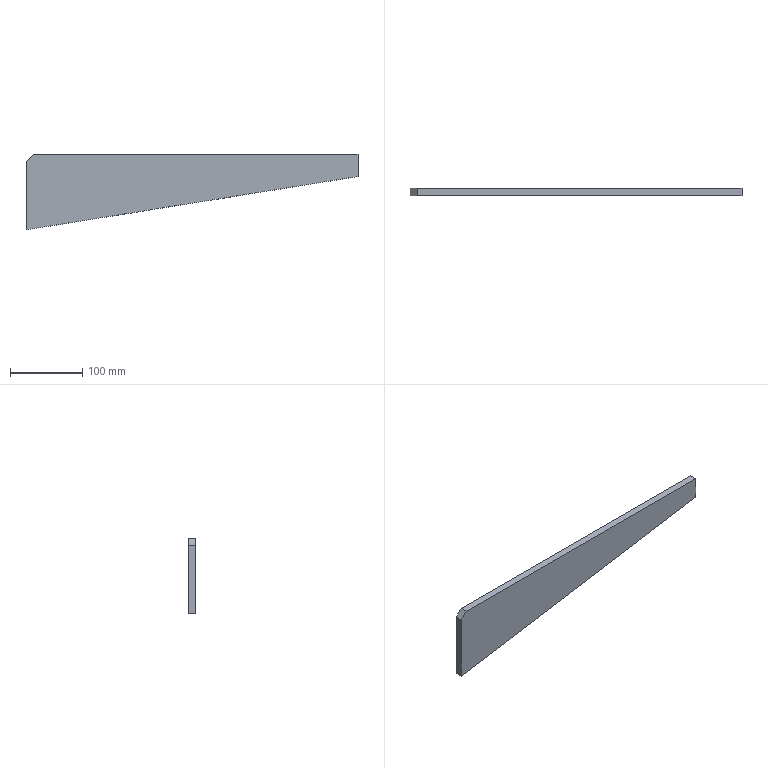Part | STEP file | Positioning_id682_x_t | 1 solid | 7 faces | box 460 x 10 x 105 mm | volume 312464 mm3 | plane 7
STEP:
#1=CARTESIAN_POINT('',(0.,0.,0.));
#2=DIRECTION('',(0.,0.,1.));
#3=DIRECTION('',(1.,0.,0.));
#4=AXIS2_PLACEMENT_3D('',#1,#2,#3);
#5=CARTESIAN_POINT('',(-1493.002,-785.,92.466));
#6=VERTEX_POINT('',#5);
#7=CARTESIAN_POINT('',(-1483.002,-785.,102.466));
#8=VERTEX_POINT('',#7);
#9=CARTESIAN_POINT('',(-1493.002,-785.,92.466));
#10=DIRECTION('',(0.7071,0.,0.7071));
#11=VECTOR('',#10,1.);
#12=LINE('',#9,#11);
#13=CARTESIAN_POINT('',(-1483.002,-790.,102.466));
#14=DIRECTION('',(0.7071,0.,-0.7071));
#15=DIRECTION('',(0.7071,0.,0.7071));
#16=AXIS2_PLACEMENT_3D('',#13,#14,#15);
#17=PLANE('',#16);
#18=CARTESIAN_POINT('',(-14.142,-5.));
#19=DIRECTION('',(1.,0.));
#20=VECTOR('',#19,1.);
#21=LINE('',#18,#20);
#22=(GEOMETRIC_REPRESENTATION_CONTEXT(2)PARAMETRIC_REPRESENTATION_CONTEXT()REPRESENTATION_CONTEXT('',''));
#23=DEFINITIONAL_REPRESENTATION('',(#21),#22);
#24=PCURVE('',#17,#23);
#25=CARTESIAN_POINT('',(-1543.002,-785.,52.466));
#26=DIRECTION('',(0.,1.,0.));
#27=DIRECTION('',(1.,0.,0.));
#28=AXIS2_PLACEMENT_3D('',#25,#26,#27);
#29=PLANE('',#28);
#30=CARTESIAN_POINT('',(50.,-40.));
#31=DIRECTION('',(0.7071,-0.7071));
#32=VECTOR('',#31,1.);
#33=LINE('',#30,#32);
#34=(GEOMETRIC_REPRESENTATION_CONTEXT(2)PARAMETRIC_REPRESENTATION_CONTEXT()REPRESENTATION_CONTEXT('',''));
#35=DEFINITIONAL_REPRESENTATION('',(#33),#34);
#36=PCURVE('',#29,#35);
#37=SURFACE_CURVE('',#12,(#24,#36),.PCURVE_S1.);
#38=EDGE_CURVE('',#6,#8,#37,.T.);
#39=ORIENTED_EDGE('',*,*,#38,.F.);
#40=CARTESIAN_POINT('',(-1493.002,-795.,92.466));
#41=VERTEX_POINT('',#40);
#42=CARTESIAN_POINT('',(-1493.002,-795.,92.466));
#43=DIRECTION('',(0.,1.,0.));
#44=VECTOR('',#43,1.);
#45=LINE('',#42,#44);
#46=CARTESIAN_POINT('',(-14.142,5.));
#47=DIRECTION('',(0.,-1.));
#48=VECTOR('',#47,1.);
#49=LINE('',#46,#48);
#50=(GEOMETRIC_REPRESENTATION_CONTEXT(2)PARAMETRIC_REPRESENTATION_CONTEXT()REPRESENTATION_CONTEXT('',''));
#51=DEFINITIONAL_REPRESENTATION('',(#49),#50);
#52=PCURVE('',#17,#51);
#53=CARTESIAN_POINT('',(-1493.002,-790.,52.466));
#54=DIRECTION('',(-1.,0.,0.));
#55=DIRECTION('',(0.,1.,0.));
#56=AXIS2_PLACEMENT_3D('',#53,#54,#55);
#57=PLANE('',#56);
#58=CARTESIAN_POINT('',(-5.,-40.));
#59=DIRECTION('',(1.,0.));
#60=VECTOR('',#59,1.);
#61=LINE('',#58,#60);
#62=(GEOMETRIC_REPRESENTATION_CONTEXT(2)PARAMETRIC_REPRESENTATION_CONTEXT()REPRESENTATION_CONTEXT('',''));
#63=DEFINITIONAL_REPRESENTATION('',(#61),#62);
#64=PCURVE('',#57,#63);
#65=SURFACE_CURVE('',#45,(#52,#64),.PCURVE_S1.);
#66=EDGE_CURVE('',#41,#6,#65,.T.);
#67=ORIENTED_EDGE('',*,*,#66,.F.);
#68=CARTESIAN_POINT('',(-1483.002,-795.,102.466));
#69=VERTEX_POINT('',#68);
#70=CARTESIAN_POINT('',(-1483.002,-795.,102.466));
#71=DIRECTION('',(-0.7071,0.,-0.7071));
#72=VECTOR('',#71,1.);
#73=LINE('',#70,#72);
#74=CARTESIAN_POINT('',(0.,5.));
#75=DIRECTION('',(-1.,0.));
#76=VECTOR('',#75,1.);
#77=LINE('',#74,#76);
#78=(GEOMETRIC_REPRESENTATION_CONTEXT(2)PARAMETRIC_REPRESENTATION_CONTEXT()REPRESENTATION_CONTEXT('',''));
#79=DEFINITIONAL_REPRESENTATION('',(#77),#78);
#80=PCURVE('',#17,#79);
#81=CARTESIAN_POINT('',(-1543.002,-795.,52.466));
#82=DIRECTION('',(0.,-1.,0.));
#83=DIRECTION('',(-1.,0.,0.));
#84=AXIS2_PLACEMENT_3D('',#81,#82,#83);
#85=PLANE('',#84);
#86=CARTESIAN_POINT('',(-60.,-50.));
#87=DIRECTION('',(0.7071,0.7071));
#88=VECTOR('',#87,1.);
#89=LINE('',#86,#88);
#90=(GEOMETRIC_REPRESENTATION_CONTEXT(2)PARAMETRIC_REPRESENTATION_CONTEXT()REPRESENTATION_CONTEXT('',''));
#91=DEFINITIONAL_REPRESENTATION('',(#89),#90);
#92=PCURVE('',#85,#91);
#93=SURFACE_CURVE('',#73,(#80,#92),.PCURVE_S1.);
#94=EDGE_CURVE('',#69,#41,#93,.T.);
#95=ORIENTED_EDGE('',*,*,#94,.F.);
#96=CARTESIAN_POINT('',(-1483.002,-785.,102.466));
#97=DIRECTION('',(0.,-1.,0.));
#98=VECTOR('',#97,1.);
#99=LINE('',#96,#98);
#100=CARTESIAN_POINT('',(0.,-5.));
#101=DIRECTION('',(0.,1.));
#102=VECTOR('',#101,1.);
#103=LINE('',#100,#102);
#104=(GEOMETRIC_REPRESENTATION_CONTEXT(2)PARAMETRIC_REPRESENTATION_CONTEXT()REPRESENTATION_CONTEXT('',''));
#105=DEFINITIONAL_REPRESENTATION('',(#103),#104);
#106=PCURVE('',#17,#105);
#107=CARTESIAN_POINT('',(-1543.002,-790.,102.466));
#108=DIRECTION('',(0.,0.,1.));
#109=DIRECTION('',(-1.,0.,0.));
#110=AXIS2_PLACEMENT_3D('',#107,#108,#109);
#111=PLANE('',#110);
#112=CARTESIAN_POINT('',(-60.,-5.));
#113=DIRECTION('',(0.,1.));
#114=VECTOR('',#113,1.);
#115=LINE('',#112,#114);
#116=(GEOMETRIC_REPRESENTATION_CONTEXT(2)PARAMETRIC_REPRESENTATION_CONTEXT()REPRESENTATION_CONTEXT('',''));
#117=DEFINITIONAL_REPRESENTATION('',(#115),#116);
#118=PCURVE('',#111,#117);
#119=SURFACE_CURVE('',#99,(#106,#118),.PCURVE_S1.);
#120=EDGE_CURVE('',#8,#69,#119,.T.);
#121=ORIENTED_EDGE('',*,*,#120,.F.);
#122=EDGE_LOOP('',(#39,#67,#95,#121));
#123=FACE_BOUND('',#122,.T.);
#124=ADVANCED_FACE('',(#123),#17,.F.);
#125=CARTESIAN_POINT('',(-1033.002,-785.,71.395));
#126=VERTEX_POINT('',#125);
#127=CARTESIAN_POINT('',(-1033.002,-795.,71.395));
#128=VERTEX_POINT('',#127);
#129=CARTESIAN_POINT('',(-1033.002,-785.,71.395));
#130=DIRECTION('',(0.,-1.,0.));
#131=VECTOR('',#130,1.);
#132=LINE('',#129,#131);
#133=CARTESIAN_POINT('',(-1493.002,-620.,-2.534));
#134=DIRECTION('',(-0.1587,0.,0.9873));
#135=DIRECTION('',(-0.9873,0.,-0.1587));
#136=AXIS2_PLACEMENT_3D('',#133,#134,#135);
#137=PLANE('',#136);
#138=CARTESIAN_POINT('',(-465.903,165.));
#139=DIRECTION('',(0.,1.));
#140=VECTOR('',#139,1.);
#141=LINE('',#138,#140);
#142=(GEOMETRIC_REPRESENTATION_CONTEXT(2)PARAMETRIC_REPRESENTATION_CONTEXT()REPRESENTATION_CONTEXT('',''));
#143=DEFINITIONAL_REPRESENTATION('',(#141),#142);
#144=PCURVE('',#137,#143);
#145=CARTESIAN_POINT('',(-1033.002,-790.,52.466));
#146=DIRECTION('',(1.,0.,0.));
#147=DIRECTION('',(0.,-1.,0.));
#148=AXIS2_PLACEMENT_3D('',#145,#146,#147);
#149=PLANE('',#148);
#150=CARTESIAN_POINT('',(-5.,-18.929));
#151=DIRECTION('',(1.,0.));
#152=VECTOR('',#151,1.);
#153=LINE('',#150,#152);
#154=(GEOMETRIC_REPRESENTATION_CONTEXT(2)PARAMETRIC_REPRESENTATION_CONTEXT()REPRESENTATION_CONTEXT('',''));
#155=DEFINITIONAL_REPRESENTATION('',(#153),#154);
#156=PCURVE('',#149,#155);
#157=SURFACE_CURVE('',#132,(#144,#156),.PCURVE_S1.);
#158=EDGE_CURVE('',#126,#128,#157,.T.);
#159=ORIENTED_EDGE('',*,*,#158,.T.);
#160=CARTESIAN_POINT('',(-1493.002,-795.,-2.534));
#161=VERTEX_POINT('',#160);
#162=CARTESIAN_POINT('',(-1033.002,-795.,71.395));
#163=DIRECTION('',(-0.9873,0.,-0.1587));
#164=VECTOR('',#163,1.);
#165=LINE('',#162,#164);
#166=CARTESIAN_POINT('',(-465.903,175.));
#167=DIRECTION('',(1.,0.));
#168=VECTOR('',#167,1.);
#169=LINE('',#166,#168);
#170=(GEOMETRIC_REPRESENTATION_CONTEXT(2)PARAMETRIC_REPRESENTATION_CONTEXT()REPRESENTATION_CONTEXT('',''));
#171=DEFINITIONAL_REPRESENTATION('',(#169),#170);
#172=PCURVE('',#137,#171);
#173=CARTESIAN_POINT('',(-510.,-18.929));
#174=DIRECTION('',(0.9873,0.1587));
#175=VECTOR('',#174,1.);
#176=LINE('',#173,#175);
#177=(GEOMETRIC_REPRESENTATION_CONTEXT(2)PARAMETRIC_REPRESENTATION_CONTEXT()REPRESENTATION_CONTEXT('',''));
#178=DEFINITIONAL_REPRESENTATION('',(#176),#177);
#179=PCURVE('',#85,#178);
#180=SURFACE_CURVE('',#165,(#172,#179),.PCURVE_S1.);
#181=EDGE_CURVE('',#128,#161,#180,.T.);
#182=ORIENTED_EDGE('',*,*,#181,.T.);
#183=CARTESIAN_POINT('',(-1493.002,-785.,-2.534));
#184=VERTEX_POINT('',#183);
#185=CARTESIAN_POINT('',(-1493.002,-795.,-2.534));
#186=DIRECTION('',(0.,1.,0.));
#187=VECTOR('',#186,1.);
#188=LINE('',#185,#187);
#189=CARTESIAN_POINT('',(0.,175.));
#190=DIRECTION('',(0.,-1.));
#191=VECTOR('',#190,1.);
#192=LINE('',#189,#191);
#193=(GEOMETRIC_REPRESENTATION_CONTEXT(2)PARAMETRIC_REPRESENTATION_CONTEXT()REPRESENTATION_CONTEXT('',''));
#194=DEFINITIONAL_REPRESENTATION('',(#192),#193);
#195=PCURVE('',#137,#194);
#196=CARTESIAN_POINT('',(-5.,55.));
#197=DIRECTION('',(1.,0.));
#198=VECTOR('',#197,1.);
#199=LINE('',#196,#198);
#200=(GEOMETRIC_REPRESENTATION_CONTEXT(2)PARAMETRIC_REPRESENTATION_CONTEXT()REPRESENTATION_CONTEXT('',''));
#201=DEFINITIONAL_REPRESENTATION('',(#199),#200);
#202=PCURVE('',#57,#201);
#203=SURFACE_CURVE('',#188,(#195,#202),.PCURVE_S1.);
#204=EDGE_CURVE('',#161,#184,#203,.T.);
#205=ORIENTED_EDGE('',*,*,#204,.T.);
#206=CARTESIAN_POINT('',(-1493.002,-785.,-2.534));
#207=DIRECTION('',(0.9873,0.,0.1587));
#208=VECTOR('',#207,1.);
#209=LINE('',#206,#208);
#210=CARTESIAN_POINT('',(0.,165.));
#211=DIRECTION('',(-1.,0.));
#212=VECTOR('',#211,1.);
#213=LINE('',#210,#212);
#214=(GEOMETRIC_REPRESENTATION_CONTEXT(2)PARAMETRIC_REPRESENTATION_CONTEXT()REPRESENTATION_CONTEXT('',''));
#215=DEFINITIONAL_REPRESENTATION('',(#213),#214);
#216=PCURVE('',#137,#215);
#217=CARTESIAN_POINT('',(50.,55.));
#218=DIRECTION('',(0.9873,-0.1587));
#219=VECTOR('',#218,1.);
#220=LINE('',#217,#219);
#221=(GEOMETRIC_REPRESENTATION_CONTEXT(2)PARAMETRIC_REPRESENTATION_CONTEXT()REPRESENTATION_CONTEXT('',''));
#222=DEFINITIONAL_REPRESENTATION('',(#220),#221);
#223=PCURVE('',#29,#222);
#224=SURFACE_CURVE('',#209,(#216,#223),.PCURVE_S1.);
#225=EDGE_CURVE('',#184,#126,#224,.T.);
#226=ORIENTED_EDGE('',*,*,#225,.T.);
#227=EDGE_LOOP('',(#159,#182,#205,#226));
#228=FACE_BOUND('',#227,.T.);
#229=ADVANCED_FACE('',(#228),#137,.F.);
#230=CARTESIAN_POINT('',(-1033.002,-785.,102.466));
#231=VERTEX_POINT('',#230);
#232=CARTESIAN_POINT('',(-1483.002,-785.,102.466));
#233=DIRECTION('',(1.,0.,0.));
#234=VECTOR('',#233,1.);
#235=LINE('',#232,#234);
#236=CARTESIAN_POINT('',(60.,-50.));
#237=DIRECTION('',(1.,0.));
#238=VECTOR('',#237,1.);
#239=LINE('',#236,#238);
#240=(GEOMETRIC_REPRESENTATION_CONTEXT(2)PARAMETRIC_REPRESENTATION_CONTEXT()REPRESENTATION_CONTEXT('',''));
#241=DEFINITIONAL_REPRESENTATION('',(#239),#240);
#242=PCURVE('',#29,#241);
#243=CARTESIAN_POINT('',(-60.,-5.));
#244=DIRECTION('',(-1.,0.));
#245=VECTOR('',#244,1.);
#246=LINE('',#243,#245);
#247=(GEOMETRIC_REPRESENTATION_CONTEXT(2)PARAMETRIC_REPRESENTATION_CONTEXT()REPRESENTATION_CONTEXT('',''));
#248=DEFINITIONAL_REPRESENTATION('',(#246),#247);
#249=PCURVE('',#111,#248);
#250=SURFACE_CURVE('',#235,(#242,#249),.PCURVE_S1.);
#251=EDGE_CURVE('',#8,#231,#250,.T.);
#252=ORIENTED_EDGE('',*,*,#251,.T.);
#253=CARTESIAN_POINT('',(-1033.002,-785.,102.466));
#254=DIRECTION('',(0.,0.,-1.));
#255=VECTOR('',#254,1.);
#256=LINE('',#253,#255);
#257=CARTESIAN_POINT('',(510.,-50.));
#258=DIRECTION('',(0.,1.));
#259=VECTOR('',#258,1.);
#260=LINE('',#257,#259);
#261=(GEOMETRIC_REPRESENTATION_CONTEXT(2)PARAMETRIC_REPRESENTATION_CONTEXT()REPRESENTATION_CONTEXT('',''));
#262=DEFINITIONAL_REPRESENTATION('',(#260),#261);
#263=PCURVE('',#29,#262);
#264=CARTESIAN_POINT('',(-5.,-50.));
#265=DIRECTION('',(0.,1.));
#266=VECTOR('',#265,1.);
#267=LINE('',#264,#266);
#268=(GEOMETRIC_REPRESENTATION_CONTEXT(2)PARAMETRIC_REPRESENTATION_CONTEXT()REPRESENTATION_CONTEXT('',''));
#269=DEFINITIONAL_REPRESENTATION('',(#267),#268);
#270=PCURVE('',#149,#269);
#271=SURFACE_CURVE('',#256,(#263,#270),.PCURVE_S1.);
#272=EDGE_CURVE('',#231,#126,#271,.T.);
#273=ORIENTED_EDGE('',*,*,#272,.T.);
#274=ORIENTED_EDGE('',*,*,#225,.F.);
#275=CARTESIAN_POINT('',(-1493.002,-785.,-2.534));
#276=DIRECTION('',(0.,0.,1.));
#277=VECTOR('',#276,1.);
#278=LINE('',#275,#277);
#279=CARTESIAN_POINT('',(50.,55.));
#280=DIRECTION('',(0.,-1.));
#281=VECTOR('',#280,1.);
#282=LINE('',#279,#281);
#283=(GEOMETRIC_REPRESENTATION_CONTEXT(2)PARAMETRIC_REPRESENTATION_CONTEXT()REPRESENTATION_CONTEXT('',''));
#284=DEFINITIONAL_REPRESENTATION('',(#282),#283);
#285=PCURVE('',#29,#284);
#286=CARTESIAN_POINT('',(5.,55.));
#287=DIRECTION('',(0.,-1.));
#288=VECTOR('',#287,1.);
#289=LINE('',#286,#288);
#290=(GEOMETRIC_REPRESENTATION_CONTEXT(2)PARAMETRIC_REPRESENTATION_CONTEXT()REPRESENTATION_CONTEXT('',''));
#291=DEFINITIONAL_REPRESENTATION('',(#289),#290);
#292=PCURVE('',#57,#291);
#293=SURFACE_CURVE('',#278,(#285,#292),.PCURVE_S1.);
#294=EDGE_CURVE('',#184,#6,#293,.T.);
#295=ORIENTED_EDGE('',*,*,#294,.T.);
#296=ORIENTED_EDGE('',*,*,#38,.T.);
#297=EDGE_LOOP('',(#252,#273,#274,#295,#296));
#298=FACE_BOUND('',#297,.T.);
#299=ADVANCED_FACE('',(#298),#29,.T.);
#300=CARTESIAN_POINT('',(-1493.002,-795.,92.466));
#301=DIRECTION('',(0.,0.,-1.));
#302=VECTOR('',#301,1.);
#303=LINE('',#300,#302);
#304=CARTESIAN_POINT('',(-5.,-40.));
#305=DIRECTION('',(0.,1.));
#306=VECTOR('',#305,1.);
#307=LINE('',#304,#306);
#308=(GEOMETRIC_REPRESENTATION_CONTEXT(2)PARAMETRIC_REPRESENTATION_CONTEXT()REPRESENTATION_CONTEXT('',''));
#309=DEFINITIONAL_REPRESENTATION('',(#307),#308);
#310=PCURVE('',#57,#309);
#311=CARTESIAN_POINT('',(-50.,-40.));
#312=DIRECTION('',(0.,1.));
#313=VECTOR('',#312,1.);
#314=LINE('',#311,#313);
#315=(GEOMETRIC_REPRESENTATION_CONTEXT(2)PARAMETRIC_REPRESENTATION_CONTEXT()REPRESENTATION_CONTEXT('',''));
#316=DEFINITIONAL_REPRESENTATION('',(#314),#315);
#317=PCURVE('',#85,#316);
#318=SURFACE_CURVE('',#303,(#310,#317),.PCURVE_S1.);
#319=EDGE_CURVE('',#41,#161,#318,.T.);
#320=ORIENTED_EDGE('',*,*,#319,.F.);
#321=ORIENTED_EDGE('',*,*,#66,.T.);
#322=ORIENTED_EDGE('',*,*,#294,.F.);
#323=ORIENTED_EDGE('',*,*,#204,.F.);
#324=EDGE_LOOP('',(#320,#321,#322,#323));
#325=FACE_BOUND('',#324,.T.);
#326=ADVANCED_FACE('',(#325),#57,.T.);
#327=CARTESIAN_POINT('',(-1033.002,-795.,102.466));
#328=VERTEX_POINT('',#327);
#329=CARTESIAN_POINT('',(-1483.002,-795.,102.466));
#330=DIRECTION('',(1.,0.,0.));
#331=VECTOR('',#330,1.);
#332=LINE('',#329,#331);
#333=CARTESIAN_POINT('',(-60.,5.));
#334=DIRECTION('',(-1.,0.));
#335=VECTOR('',#334,1.);
#336=LINE('',#333,#335);
#337=(GEOMETRIC_REPRESENTATION_CONTEXT(2)PARAMETRIC_REPRESENTATION_CONTEXT()REPRESENTATION_CONTEXT('',''));
#338=DEFINITIONAL_REPRESENTATION('',(#336),#337);
#339=PCURVE('',#111,#338);
#340=CARTESIAN_POINT('',(-60.,-50.));
#341=DIRECTION('',(-1.,0.));
#342=VECTOR('',#341,1.);
#343=LINE('',#340,#342);
#344=(GEOMETRIC_REPRESENTATION_CONTEXT(2)PARAMETRIC_REPRESENTATION_CONTEXT()REPRESENTATION_CONTEXT('',''));
#345=DEFINITIONAL_REPRESENTATION('',(#343),#344);
#346=PCURVE('',#85,#345);
#347=SURFACE_CURVE('',#332,(#339,#346),.PCURVE_S1.);
#348=EDGE_CURVE('',#69,#328,#347,.T.);
#349=ORIENTED_EDGE('',*,*,#348,.T.);
#350=CARTESIAN_POINT('',(-1033.002,-795.,102.466));
#351=DIRECTION('',(0.,1.,0.));
#352=VECTOR('',#351,1.);
#353=LINE('',#350,#352);
#354=CARTESIAN_POINT('',(-510.,5.));
#355=DIRECTION('',(0.,-1.));
#356=VECTOR('',#355,1.);
#357=LINE('',#354,#356);
#358=(GEOMETRIC_REPRESENTATION_CONTEXT(2)PARAMETRIC_REPRESENTATION_CONTEXT()REPRESENTATION_CONTEXT('',''));
#359=DEFINITIONAL_REPRESENTATION('',(#357),#358);
#360=PCURVE('',#111,#359);
#361=CARTESIAN_POINT('',(5.,-50.));
#362=DIRECTION('',(-1.,0.));
#363=VECTOR('',#362,1.);
#364=LINE('',#361,#363);
#365=(GEOMETRIC_REPRESENTATION_CONTEXT(2)PARAMETRIC_REPRESENTATION_CONTEXT()REPRESENTATION_CONTEXT('',''));
#366=DEFINITIONAL_REPRESENTATION('',(#364),#365);
#367=PCURVE('',#149,#366);
#368=SURFACE_CURVE('',#353,(#360,#367),.PCURVE_S1.);
#369=EDGE_CURVE('',#328,#231,#368,.T.);
#370=ORIENTED_EDGE('',*,*,#369,.T.);
#371=ORIENTED_EDGE('',*,*,#251,.F.);
#372=ORIENTED_EDGE('',*,*,#120,.T.);
#373=EDGE_LOOP('',(#349,#370,#371,#372));
#374=FACE_BOUND('',#373,.T.);
#375=ADVANCED_FACE('',(#374),#111,.T.);
#376=CARTESIAN_POINT('',(-1033.002,-795.,71.395));
#377=DIRECTION('',(0.,0.,1.));
#378=VECTOR('',#377,1.);
#379=LINE('',#376,#378);
#380=CARTESIAN_POINT('',(-510.,-18.929));
#381=DIRECTION('',(0.,-1.));
#382=VECTOR('',#381,1.);
#383=LINE('',#380,#382);
#384=(GEOMETRIC_REPRESENTATION_CONTEXT(2)PARAMETRIC_REPRESENTATION_CONTEXT()REPRESENTATION_CONTEXT('',''));
#385=DEFINITIONAL_REPRESENTATION('',(#383),#384);
#386=PCURVE('',#85,#385);
#387=CARTESIAN_POINT('',(5.,-18.929));
#388=DIRECTION('',(0.,-1.));
#389=VECTOR('',#388,1.);
#390=LINE('',#387,#389);
#391=(GEOMETRIC_REPRESENTATION_CONTEXT(2)PARAMETRIC_REPRESENTATION_CONTEXT()REPRESENTATION_CONTEXT('',''));
#392=DEFINITIONAL_REPRESENTATION('',(#390),#391);
#393=PCURVE('',#149,#392);
#394=SURFACE_CURVE('',#379,(#386,#393),.PCURVE_S1.);
#395=EDGE_CURVE('',#128,#328,#394,.T.);
#396=ORIENTED_EDGE('',*,*,#395,.T.);
#397=ORIENTED_EDGE('',*,*,#348,.F.);
#398=ORIENTED_EDGE('',*,*,#94,.T.);
#399=ORIENTED_EDGE('',*,*,#319,.T.);
#400=ORIENTED_EDGE('',*,*,#181,.F.);
#401=EDGE_LOOP('',(#396,#397,#398,#399,#400));
#402=FACE_BOUND('',#401,.T.);
#403=ADVANCED_FACE('',(#402),#85,.T.);
#404=ORIENTED_EDGE('',*,*,#369,.F.);
#405=ORIENTED_EDGE('',*,*,#395,.F.);
#406=ORIENTED_EDGE('',*,*,#158,.F.);
#407=ORIENTED_EDGE('',*,*,#272,.F.);
#408=EDGE_LOOP('',(#404,#405,#406,#407));
#409=FACE_BOUND('',#408,.T.);
#410=ADVANCED_FACE('',(#409),#149,.T.);
#411=CLOSED_SHELL('',(#124,#229,#299,#326,#375,#403,#410));
#412=MANIFOLD_SOLID_BREP('',#411);
#413=(LENGTH_UNIT()NAMED_UNIT(*)SI_UNIT(.MILLI.,.METRE.));
#414=UNCERTAINTY_MEASURE_WITH_UNIT(LENGTH_MEASURE(0.0000001),#413,'','');
#415=(NAMED_UNIT(*)PLANE_ANGLE_UNIT()SI_UNIT($,.RADIAN.));
#416=(NAMED_UNIT(*)SI_UNIT($,.STERADIAN.)SOLID_ANGLE_UNIT());
#417=(GEOMETRIC_REPRESENTATION_CONTEXT(3)GLOBAL_UNCERTAINTY_ASSIGNED_CONTEXT((#414))GLOBAL_UNIT_ASSIGNED_CONTEXT((#413,#415,#416))REPRESENTATION_CONTEXT('',''));
#418=ADVANCED_BREP_SHAPE_REPRESENTATION('',(#4,#412),#417);